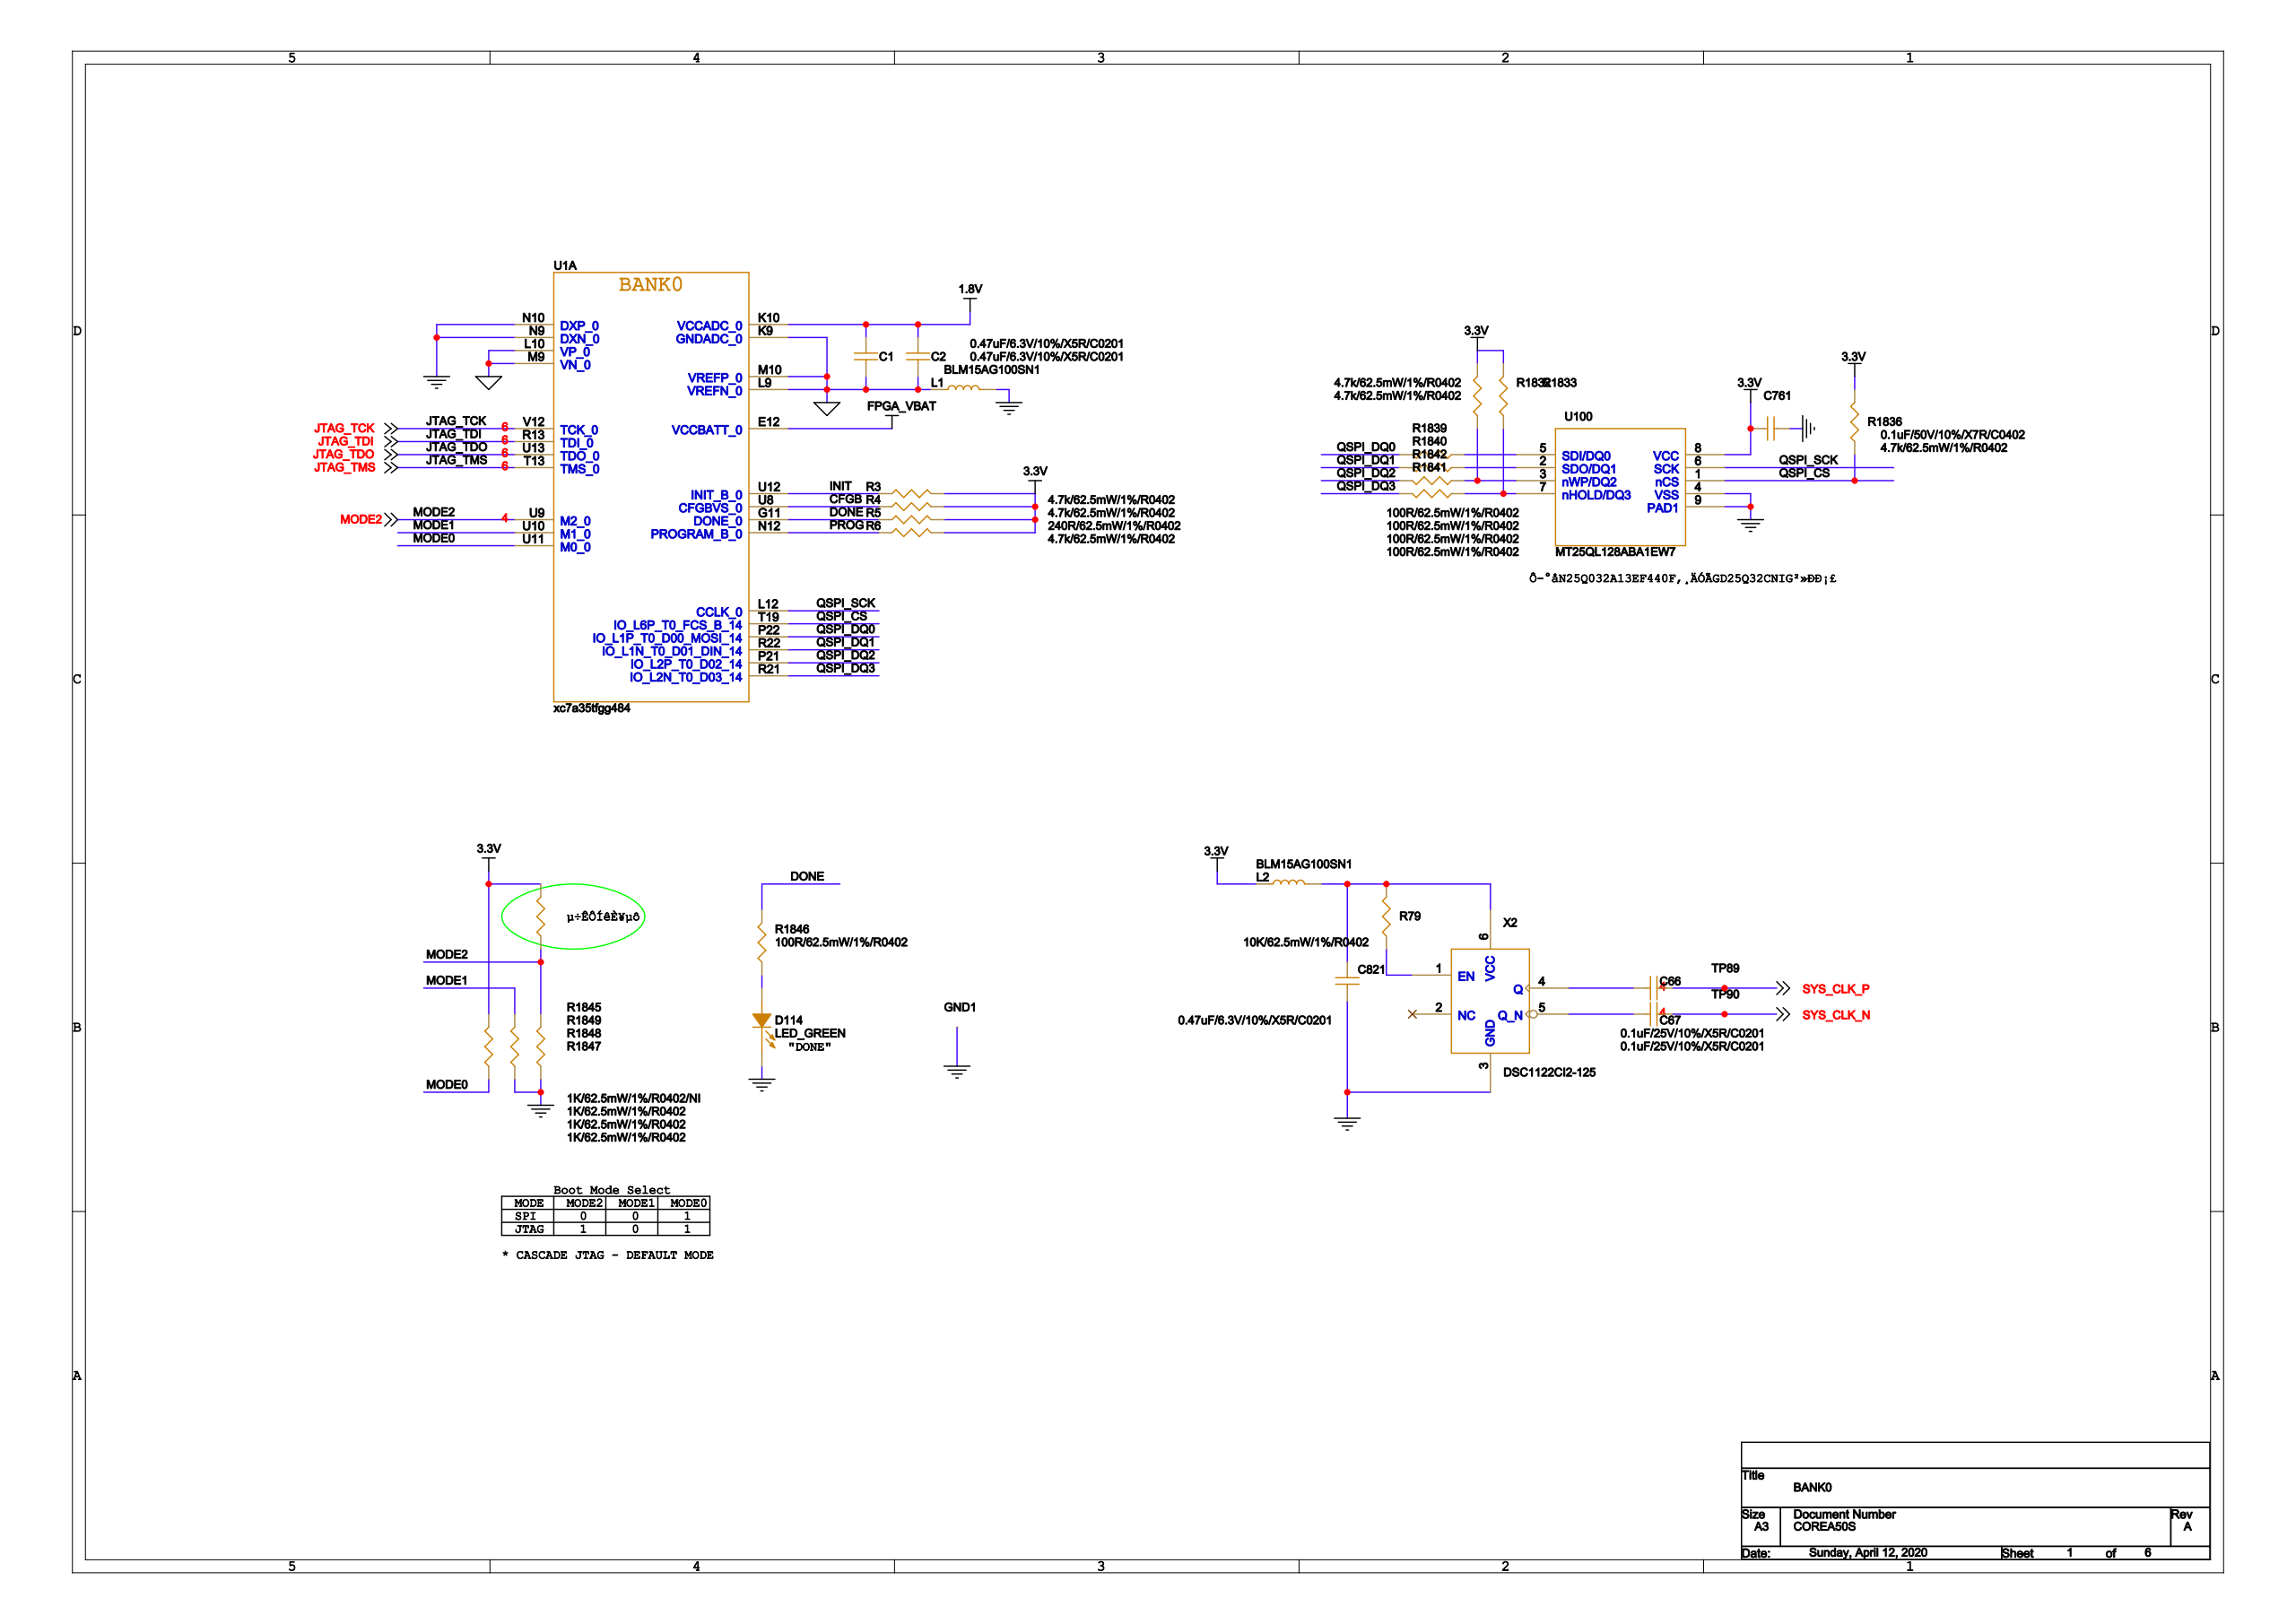Circuit board | Cadence Allegro | 202 parts | 354 nets | one sheet of the schematic
Parts on this sheet (reference | value | footprint):
C2 | 0.47uF/6.3V/10%/X5R/C0201 | 0201
C66 | 0.1uF/25V/10%/X5R/C0201 | 0201
C67 | 0.1uF/25V/10%/X5R/C0201 | 0201
C761 | 0.1uF/50V/10%/X7R/C0402 | 0402
C821 | 0.47uF/6.3V/10%/X5R/C0201 | 0201
D114 | LED_GREEN | LED0805
L1 | BLM15AG100SN1 | 0402
L2 | BLM15AG100SN1 | 0402
R3 | 4.7k/62.5mW/1%/R0402 | 0402
R4 | 4.7k/62.5mW/1%/R0402 | 0402
R5 | 240R/62.5mW/1%/R0402 | 0402
R6 | 4.7k/62.5mW/1%/R0402 | 0402
R79 | 10K/62.5mW/1%/R0402 | 0402
R1832 | 4.7k/62.5mW/1%/R0402 | 0402
R1833 | 4.7k/62.5mW/1%/R0402 | 0402
R1836 | 4.7k/62.5mW/1%/R0402 | 0402
R1839 | 100R/62.5mW/1%/R0402 | 0402
R1840 | 100R/62.5mW/1%/R0402 | 0402
R1841 | 100R/62.5mW/1%/R0402 | 0402
R1842 | 100R/62.5mW/1%/R0402 | 0402
R1845 | 1K/62.5mW/1%/R0402/NI | 0402
R1846 | 100R/62.5mW/1%/R0402 | 0402
R1847 | 1K/62.5mW/1%/R0402 | 0402
R1848 | 1K/62.5mW/1%/R0402 | 0402
R1849 | 1K/62.5mW/1%/R0402 | 0402
TP89 | TEST POINT A | TEST_12MM
TP90 | TEST POINT A | TEST_12MM
U1 | xc7a35tfgg484 | FGG484_23X23
U100 | MT25QL128ABA1EW7 | WPDFN-8_6X5
X2 | DSC1122CI2-125 | VDFN-3225
Nets of these parts (net: part-pin ...):
GND: C761-1 C821-2 D114-2 L1-2 R1848-2 R1849-2 U100-4 U100-9 X2-3 U1-A3 U1-L2 U1-N9 U1-N10
QSPI_CS: R1836-2 U100-1 U1-T19
N26203831: R1833-2 R1841-1 U100-7
N26203829: R1832-2 R1842-1 U100-3
QSPI_SCK: U100-6 U1-L12
N26203907: R1839-1 U100-5
N26203934: R1840-1 U100-2
3.3V: C761-2 L2-1 R3-1 R4-1 R5-1 R6-1 R1832-1 R1833-1 R1836-1 R1845-1 R1847-1 U100-8 U1-C1 U1-R5
CFGB: R4-2 U1-U8
DONE: R5-2 R1846-2 U1-G11
AGND: C2-2 L1-1 U1-K9 U1-L9 U1-L10 U1-M9 U1-M10
INIT: R3-2 U1-U12
QSPI_DQ1: R1840-2 U1-R22
QSPI_DQ0: R1839-2 U1-P22
QSPI_DQ3: R1841-2 U1-R21
QSPI_DQ2: R1842-2 U1-P21
MODE0: R1847-2 U1-U11
MODE1: R1848-1 U1-U10
MODE2: R1845-2 R1849-1 U1-U9
PROG: R6-2 U1-N12
JTAG_TCK: U1-V12
JTAG_TDI: U1-R13
JTAG_TDO: U1-U13
JTAG_TMS: U1-T13
1.8V: C2-1 U1-K10
FPGA_VBAT: U1-E12
SYS_CLK_N: C67-1 TP90-1
SYS_CLK_P: C66-1 TP89-1
N26427357: R79-1 X2-1
N26427318: C821-1 L2-2 R79-2 X2-6
N26436885: C66-2 X2-4
N26436888: C67-2 X2-5
N26204114: D114-1 R1846-1